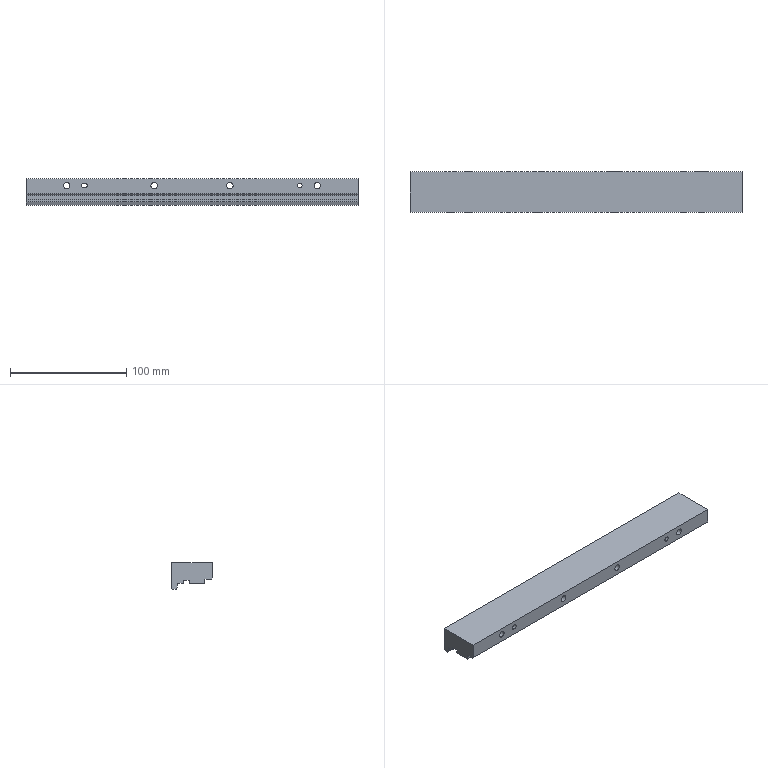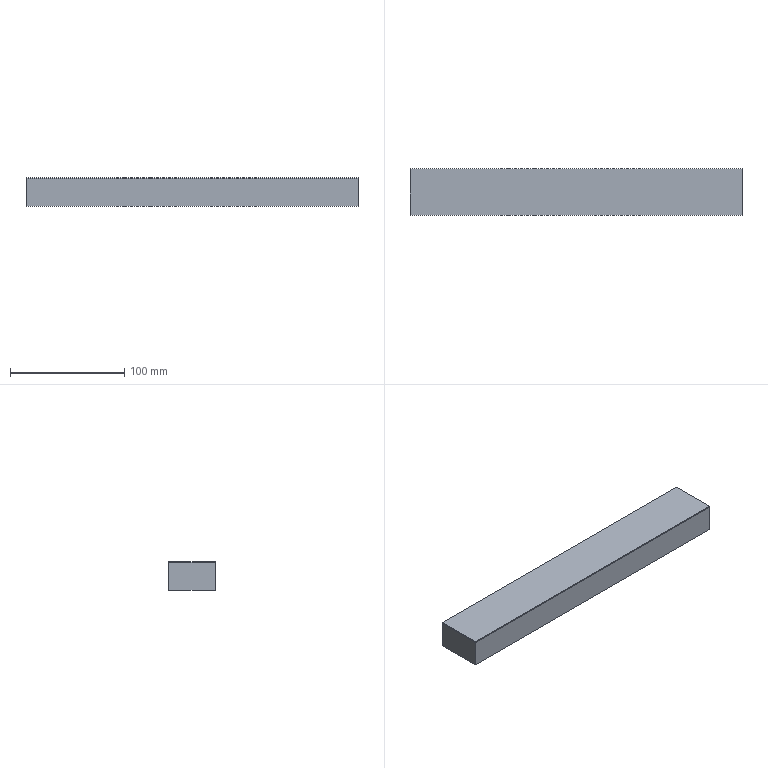CAM job | NX | 3-axis milling | part box 285 x 35 x 22.9 mm | stock box 291 x 41 x 24.9 mm
Tools:
number,name,description,diameter,corner_radius,flute_length,length,flutes
1,D50,Milling Tool-5 Parameters,50.0,0.0,50.0,75.0,2
3,D10,Milling Tool-5 Parameters,10.0,0.0,50.0,75.0,2
4,D10JING,Milling Tool-5 Parameters,10.0,0.0,50.0,75.0,2
2,D6A45,Milling Tool-5 Parameters,6.0,0.0,3.0,3.0,2
8,D6,Milling Tool-5 Parameters,6.0,0.0,50.0,75.0,2
10,D4,Milling Tool-5 Parameters,4.0,0.0,50.0,75.0,2
20,D6R0.5,Milling Tool-5 Parameters,6.0,0.5,50.0,75.0,2
Operations:
program,operation,operation_type,tool,method,geometry_group,spindle_rpm,surface_speed,feed_per_tooth,feed_cut,feed_plunge,cut_length_mm,path_length_mm,cut_time_min,machine_time_min
1-293-40-25毛胚,FLOOR_WALL,VolumeBased25DMillingOperation,D50,METHOD,A,6500.0,1286.0,0.0962,1250.0,100.0,353.0,407.0,0.2824,0.2878
1-293-40-25毛胚,ZLEVEL_PROFILE,ZLevelMilling,D10,METHOD,A,7000.0,219.0,0.2143,3000.0,1000.0,15563.435,15643.335,5.22,5.228
1-293-40-25毛胚,ZLEVEL_PROFILE_COPY_COPY_1_COPY_COPY_COPY_1,ZLevelMilling,D10JING,METHOD,A,7000.0,219.0,0.0714,1000.0,100.0,1349.097,1455.116,1.349,1.36
1-293-40-25毛胚,ZLEVEL_PROFILE_COPY_1_COPY_COPY_COPY_COPY_2_COPY,ZLevelMilling,D6A45,METHOD,A,7000.0,131.0,0.0714,1000.0,1000.0,649.121,711.121,0.6491,0.6553
2-293-40-25毛胚,FLOOR_WALL_COPY,VolumeBased25DMillingOperation,D50,METHOD,B,6500.0,1286.0,0.0962,1250.0,100.0,706.0,1159,0.5648,0.6101
2-293-40-25毛胚,FLOOR_WALL_1,VolumeBased25DMillingOperation,D10,METHOD,B,7000.0,219.0,0.2143,3000.0,1000.0,2085.061,2156.361,0.699,0.7062
2-293-40-25毛胚,FLOOR_WALL_1_COPY,VolumeBased25DMillingOperation,D10,METHOD,B,7000.0,219.0,0.2143,3000.0,1000.0,7115.15,7178.85,2.376,2.382
2-293-40-25毛胚,FLOOR_WALL_1_COPY_1_1,VolumeBased25DMillingOperation,D6,METHOD,B,7000.0,87.0,0.0714,1000.0,100.0,4138.709,4943.577,4.139,4.239
2-293-40-25毛胚,FLOOR_WALL_1_1,VolumeBased25DMillingOperation,D4,METHOD,B,7000.0,87.0,0.1429,2000.0,1000.0,4085.9,4159.6,2.064,2.072
2-293-40-25毛胚,FLOOR_WALL_1_COPY_1,VolumeBased25DMillingOperation,D4,METHOD,B,7000.0,87.0,0.0714,1000.0,100.0,1181.599,1257.999,1.182,1.189
2-293-40-25毛胚,ZLEVEL_PROFILE_COPY_COPY_1_COPY_COPY_COPY_1_COPY_COPY,ZLevelMilling,D6R0.5,METHOD,B,7000.0,131.0,0.2143,3000.0,1000.0,11157.415,11221.005,3.72,3.726
2-293-40-25毛胚,ZLEVEL_PROFILE_COPY_1_COPY_COPY_COPY_COPY_2_COPY_COPY_COPY_COPY,ZLevelMilling,D6A45,METHOD,B,7000.0,131.0,0.0714,1000.0,1000.0,305.652,368.652,0.3057,0.312
2-293-40-25毛胚,ZLEVEL_PROFILE_COPY_1_COPY_COPY_COPY_COPY_2_COPY_COPY,ZLevelMilling,D6A45,METHOD,B,7000.0,131.0,0.0714,1000.0,1000.0,903.734,1338.842,0.9037,0.9472
2-293-40-25毛胚,ZLEVEL_PROFILE_COPY_1_COPY_COPY_COPY_COPY_2_COPY_COPY_COPY,ZLevelMilling,D6A45,METHOD,B,7000.0,131.0,0.0714,1000.0,1000.0,301.898,383.498,0.3019,0.3101